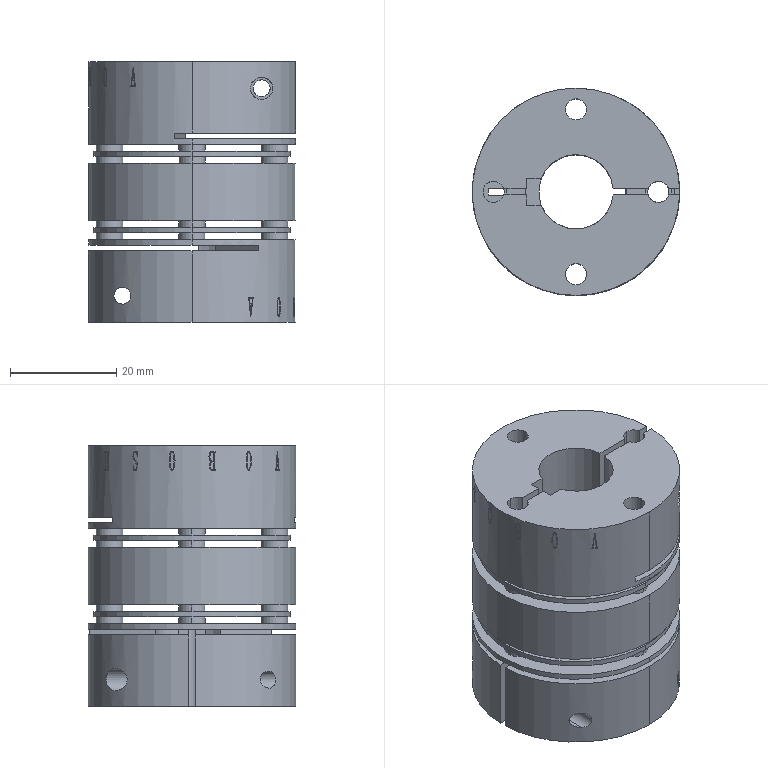Part | SolidWorks | features ICE 15, RevCut 7, CirPattern 3, Emboss 2, MirrorPattern 1, Revolution 1 | 1 solid | 412 faces | box 39 x 39 x 49 mm | volume 38785 mm3 | plane 161 | spline 130 | cylinder 121 | commonest cylinder face diameters 5 x32 4 x21 39 x19 39.02 x12 3.2 x8 4.4 x8